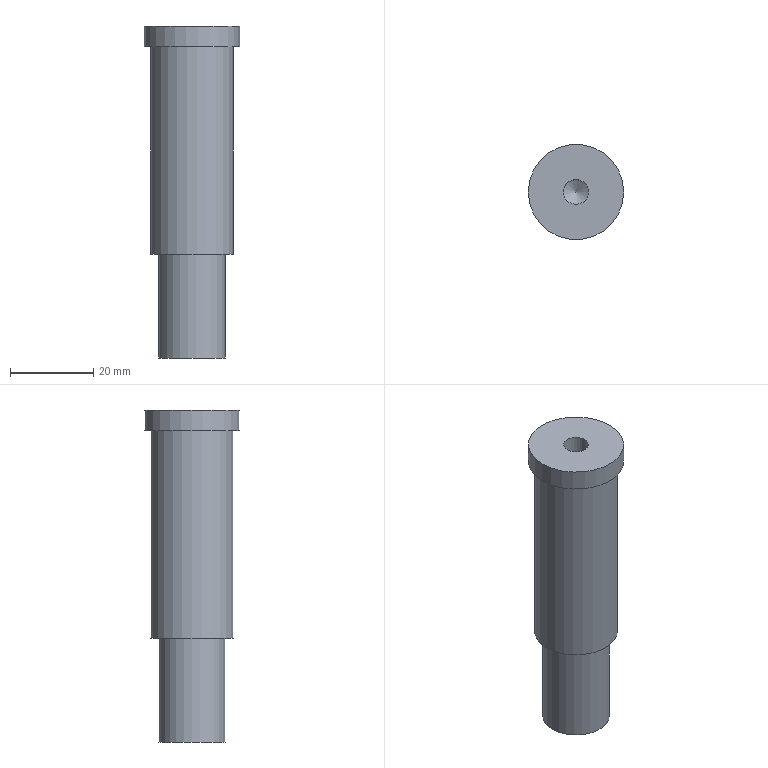Part | NX | features solid 2 | 1 solid | 9 faces | box 23 x 23 x 80 mm | volume 22491 mm3 | cylinder 4 | plane 4 | cone 1 | commonest cylinder face diameters 6 x1 16.1 x1 20 x1 23 x1
STEP:
#1=CARTESIAN_POINT('',(-111.848,-197.,136.));
#2=VERTEX_POINT('',#1);
#3=CARTESIAN_POINT('',(-121.848,-197.,136.));
#4=DIRECTION('',(0.,0.,1.));
#5=DIRECTION('',(1.,0.,0.));
#6=AXIS2_PLACEMENT_3D('',#3,#4,#5);
#7=CIRCLE('',#6,10.);
#8=EDGE_CURVE('',#2,#2,#7,.T.);
#9=ORIENTED_EDGE('',*,*,#8,.T.);
#10=EDGE_LOOP('',(#9));
#11=FACE_BOUND('',#10,.T.);
#12=CARTESIAN_POINT('',(-111.848,-197.,186.));
#13=VERTEX_POINT('',#12);
#14=CARTESIAN_POINT('',(-121.848,-197.,186.));
#15=DIRECTION('',(0.,0.,1.));
#16=DIRECTION('',(1.,0.,0.));
#17=AXIS2_PLACEMENT_3D('',#14,#15,#16);
#18=CIRCLE('',#17,10.);
#19=EDGE_CURVE('',#13,#13,#18,.T.);
#20=ORIENTED_EDGE('',*,*,#19,.F.);
#21=EDGE_LOOP('',(#20));
#22=FACE_BOUND('',#21,.T.);
#23=CARTESIAN_POINT('',(-121.848,-197.,191.));
#24=DIRECTION('',(0.,0.,-1.));
#25=DIRECTION('',(-1.,0.,0.));
#26=AXIS2_PLACEMENT_3D('',#23,#24,#25);
#27=CYLINDRICAL_SURFACE('',#26,10.);
#28=ADVANCED_FACE('',(#11,#22),#27,.T.);
#29=CARTESIAN_POINT('',(-113.798,-197.,136.));
#30=VERTEX_POINT('',#29);
#31=CARTESIAN_POINT('',(-121.848,-197.,136.));
#32=DIRECTION('',(0.,0.,1.));
#33=DIRECTION('',(1.,0.,0.));
#34=AXIS2_PLACEMENT_3D('',#31,#32,#33);
#35=CIRCLE('',#34,8.05);
#36=EDGE_CURVE('',#30,#30,#35,.T.);
#37=ORIENTED_EDGE('',*,*,#36,.T.);
#38=EDGE_LOOP('',(#37));
#39=FACE_BOUND('',#38,.T.);
#40=ORIENTED_EDGE('',*,*,#8,.F.);
#41=EDGE_LOOP('',(#40));
#42=FACE_BOUND('',#41,.T.);
#43=CARTESIAN_POINT('',(-121.848,-197.,136.));
#44=DIRECTION('',(0.,0.,1.));
#45=DIRECTION('',(1.,0.,0.));
#46=AXIS2_PLACEMENT_3D('',#43,#44,#45);
#47=PLANE('',#46);
#48=ADVANCED_FACE('',(#39,#42),#47,.F.);
#49=CARTESIAN_POINT('',(-110.348,-197.,186.));
#50=VERTEX_POINT('',#49);
#51=CARTESIAN_POINT('',(-121.848,-197.,186.));
#52=DIRECTION('',(0.,0.,1.));
#53=DIRECTION('',(1.,0.,0.));
#54=AXIS2_PLACEMENT_3D('',#51,#52,#53);
#55=CIRCLE('',#54,11.5);
#56=EDGE_CURVE('',#50,#50,#55,.T.);
#57=ORIENTED_EDGE('',*,*,#56,.F.);
#58=EDGE_LOOP('',(#57));
#59=FACE_BOUND('',#58,.T.);
#60=ORIENTED_EDGE('',*,*,#19,.T.);
#61=EDGE_LOOP('',(#60));
#62=FACE_BOUND('',#61,.T.);
#63=CARTESIAN_POINT('',(-121.848,-197.,186.));
#64=DIRECTION('',(0.,0.,1.));
#65=DIRECTION('',(1.,0.,0.));
#66=AXIS2_PLACEMENT_3D('',#63,#64,#65);
#67=PLANE('',#66);
#68=ADVANCED_FACE('',(#59,#62),#67,.F.);
#69=ORIENTED_EDGE('',*,*,#56,.T.);
#70=EDGE_LOOP('',(#69));
#71=FACE_BOUND('',#70,.T.);
#72=CARTESIAN_POINT('',(-110.348,-197.,191.));
#73=VERTEX_POINT('',#72);
#74=CARTESIAN_POINT('',(-121.848,-197.,191.));
#75=DIRECTION('',(0.,0.,1.));
#76=DIRECTION('',(1.,0.,0.));
#77=AXIS2_PLACEMENT_3D('',#74,#75,#76);
#78=CIRCLE('',#77,11.5);
#79=EDGE_CURVE('',#73,#73,#78,.T.);
#80=ORIENTED_EDGE('',*,*,#79,.F.);
#81=EDGE_LOOP('',(#80));
#82=FACE_BOUND('',#81,.T.);
#83=CARTESIAN_POINT('',(-121.848,-197.,186.));
#84=DIRECTION('',(0.,0.,1.));
#85=DIRECTION('',(1.,0.,0.));
#86=AXIS2_PLACEMENT_3D('',#83,#84,#85);
#87=CYLINDRICAL_SURFACE('',#86,11.5);
#88=ADVANCED_FACE('',(#71,#82),#87,.T.);
#89=CARTESIAN_POINT('',(-124.848,-197.,191.));
#90=VERTEX_POINT('',#89);
#91=CARTESIAN_POINT('',(-121.848,-197.,191.));
#92=DIRECTION('',(0.,0.,-1.));
#93=DIRECTION('',(-1.,0.,0.));
#94=AXIS2_PLACEMENT_3D('',#91,#92,#93);
#95=CIRCLE('',#94,3.);
#96=EDGE_CURVE('',#90,#90,#95,.T.);
#97=ORIENTED_EDGE('',*,*,#96,.T.);
#98=EDGE_LOOP('',(#97));
#99=FACE_BOUND('',#98,.T.);
#100=ORIENTED_EDGE('',*,*,#79,.T.);
#101=EDGE_LOOP('',(#100));
#102=FACE_BOUND('',#101,.T.);
#103=CARTESIAN_POINT('',(-121.848,-197.,191.));
#104=DIRECTION('',(0.,0.,1.));
#105=DIRECTION('',(1.,0.,0.));
#106=AXIS2_PLACEMENT_3D('',#103,#104,#105);
#107=PLANE('',#106);
#108=ADVANCED_FACE('',(#99,#102),#107,.T.);
#109=CARTESIAN_POINT('',(-113.798,-197.,111.));
#110=VERTEX_POINT('',#109);
#111=CARTESIAN_POINT('',(-121.848,-197.,111.));
#112=DIRECTION('',(0.,0.,1.));
#113=DIRECTION('',(1.,0.,0.));
#114=AXIS2_PLACEMENT_3D('',#111,#112,#113);
#115=CIRCLE('',#114,8.05);
#116=EDGE_CURVE('',#110,#110,#115,.T.);
#117=ORIENTED_EDGE('',*,*,#116,.T.);
#118=EDGE_LOOP('',(#117));
#119=FACE_BOUND('',#118,.T.);
#120=ORIENTED_EDGE('',*,*,#36,.F.);
#121=EDGE_LOOP('',(#120));
#122=FACE_BOUND('',#121,.T.);
#123=CARTESIAN_POINT('',(-121.848,-197.,111.));
#124=DIRECTION('',(0.,0.,1.));
#125=DIRECTION('',(1.,0.,0.));
#126=AXIS2_PLACEMENT_3D('',#123,#124,#125);
#127=CYLINDRICAL_SURFACE('',#126,8.05);
#128=ADVANCED_FACE('',(#119,#122),#127,.T.);
#129=ORIENTED_EDGE('',*,*,#116,.F.);
#130=EDGE_LOOP('',(#129));
#131=FACE_BOUND('',#130,.T.);
#132=CARTESIAN_POINT('',(-121.848,-197.,111.));
#133=DIRECTION('',(0.,0.,1.));
#134=DIRECTION('',(1.,0.,0.));
#135=AXIS2_PLACEMENT_3D('',#132,#133,#134);
#136=PLANE('',#135);
#137=ADVANCED_FACE('',(#131),#136,.F.);
#138=CARTESIAN_POINT('',(-124.848,-197.,178.));
#139=VERTEX_POINT('',#138);
#140=CARTESIAN_POINT('',(-121.848,-197.,178.));
#141=DIRECTION('',(0.,0.,-1.));
#142=DIRECTION('',(-1.,0.,0.));
#143=AXIS2_PLACEMENT_3D('',#140,#141,#142);
#144=CIRCLE('',#143,3.);
#145=EDGE_CURVE('',#139,#139,#144,.T.);
#146=ORIENTED_EDGE('',*,*,#145,.F.);
#147=EDGE_LOOP('',(#146));
#148=FACE_BOUND('',#147,.T.);
#149=CARTESIAN_POINT('',(-121.848,-197.,176.268));
#150=VERTEX_POINT('',#149);
#151=VERTEX_LOOP('',#150);
#152=FACE_BOUND('',#151,.T.);
#153=CARTESIAN_POINT('',(-121.848,-197.,178.));
#154=DIRECTION('',(0.,0.,1.));
#155=DIRECTION('',(1.,0.,0.));
#156=AXIS2_PLACEMENT_3D('',#153,#154,#155);
#157=CONICAL_SURFACE('',#156,3.,1.047);
#158=ADVANCED_FACE('',(#148,#152),#157,.F.);
#159=ORIENTED_EDGE('',*,*,#145,.T.);
#160=EDGE_LOOP('',(#159));
#161=FACE_BOUND('',#160,.T.);
#162=ORIENTED_EDGE('',*,*,#96,.F.);
#163=EDGE_LOOP('',(#162));
#164=FACE_BOUND('',#163,.T.);
#165=CARTESIAN_POINT('',(-121.848,-197.,191.));
#166=DIRECTION('',(0.,0.,-1.));
#167=DIRECTION('',(-1.,0.,0.));
#168=AXIS2_PLACEMENT_3D('',#165,#166,#167);
#169=CYLINDRICAL_SURFACE('',#168,3.);
#170=ADVANCED_FACE('',(#161,#164),#169,.F.);
#171=CLOSED_SHELL('',(#28,#48,#68,#88,#108,#128,#137,#158,#170));
#172=MANIFOLD_SOLID_BREP('',#171);
#173=(LENGTH_UNIT()NAMED_UNIT(*)SI_UNIT(.MILLI.,.METRE.));
#174=UNCERTAINTY_MEASURE_WITH_UNIT(LENGTH_MEASURE(0.00001),#173,'','');
#175=(NAMED_UNIT(*)PLANE_ANGLE_UNIT()SI_UNIT($,.RADIAN.));
#176=(NAMED_UNIT(*)SI_UNIT($,.STERADIAN.)SOLID_ANGLE_UNIT());
#177=(GEOMETRIC_REPRESENTATION_CONTEXT(3)GLOBAL_UNCERTAINTY_ASSIGNED_CONTEXT((#174))GLOBAL_UNIT_ASSIGNED_CONTEXT((#173,#175,#176))REPRESENTATION_CONTEXT('',''));
#178=ADVANCED_BREP_SHAPE_REPRESENTATION('',(#172),#177);